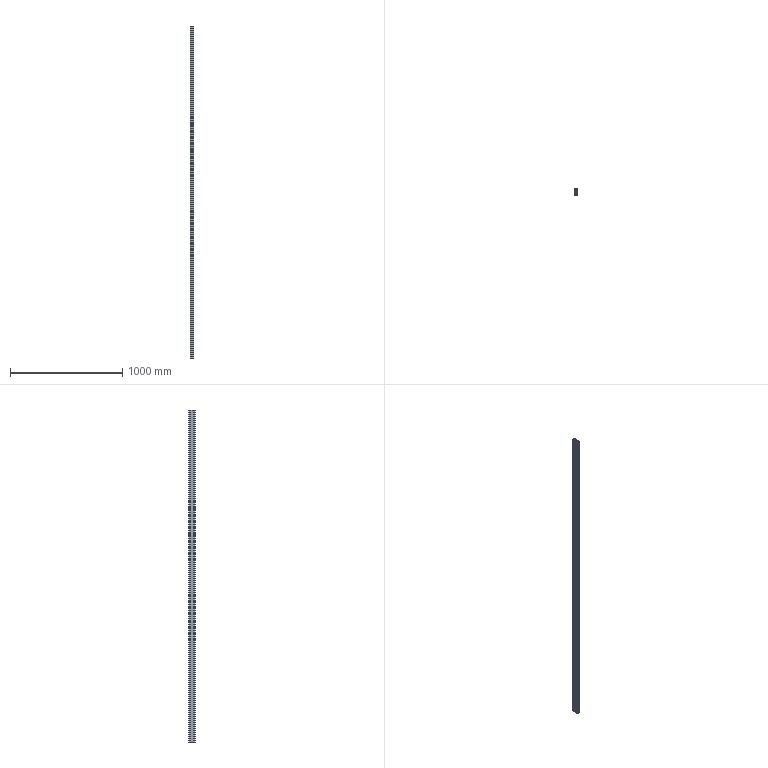Part | STEP file | ASND-0110-5.3 | 1 solid | 124 faces | box 30 x 60 x 2960 mm | volume 1832214 mm3 | plane 94 | cylinder 30 | commonest cylinder face diameters 0.6 x12 2 x4 4 x4 4.2 x4 6.8 x4 12 x2